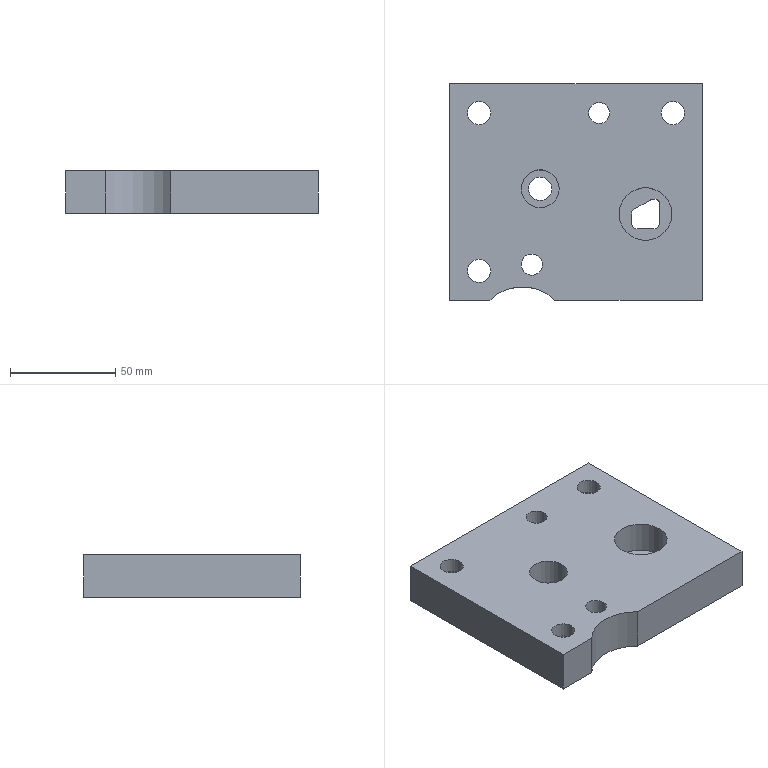Part | STEP file | 402_id34_x_t | 1 solid | 38 faces | box 120 x 103 x 20 mm | volume 217501 mm3 | plane 19 | cylinder 19 | commonest cylinder face diameters 5 x3 11 x3 17 x3 10 x2 12 x2 2 x1